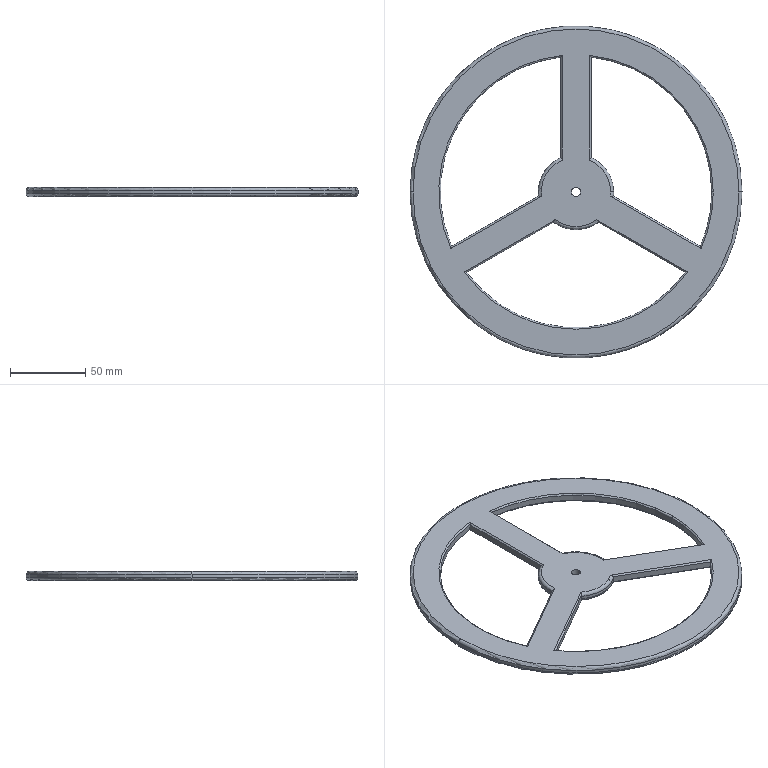Part | SolidWorks | features Fillet 3, Chamfer 1, Extrusion 1, ICE 1 | 1 solid | 51 faces | box 220.16 x 220.16 x 6 mm | volume 108989 mm3 | torus 20 | plane 19 | cylinder 12 | commonest cylinder face diameters 50 x4 180 x4 6 x2 220.16 x2